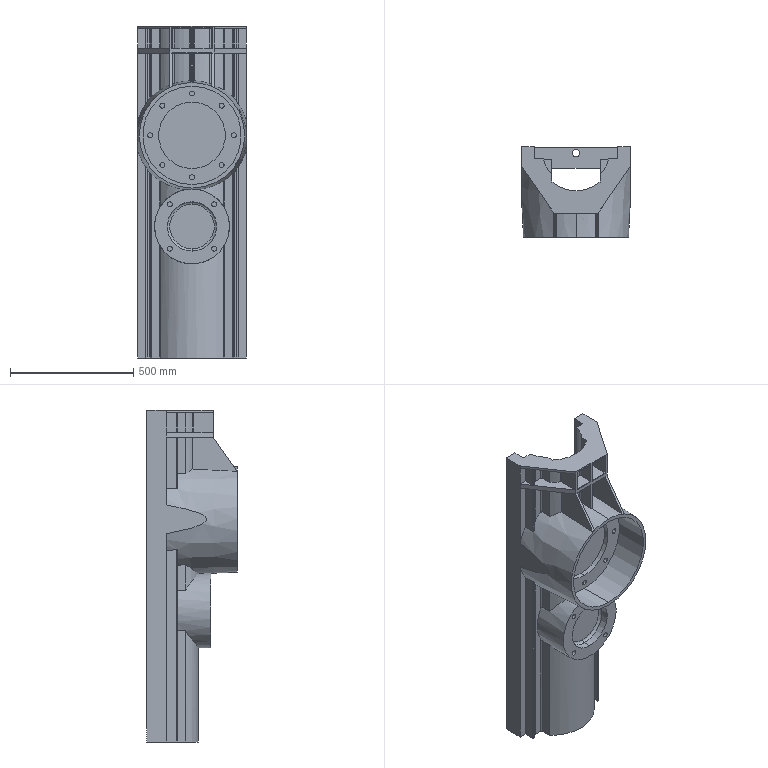Part | SolidWorks | features ICE 24, Fillet 8, MirrorPattern 4, CirPattern 2, Extrusion 1 | 1 solid | 262 faces | box 440 x 367.835 x 1348 mm | volume 54378577 mm3 | plane 129 | cylinder 128 | cone 3 | torus 2 | commonest cylinder face diameters 16 x32 10 x27 20 x24 4 x22 360 x11 30 x2